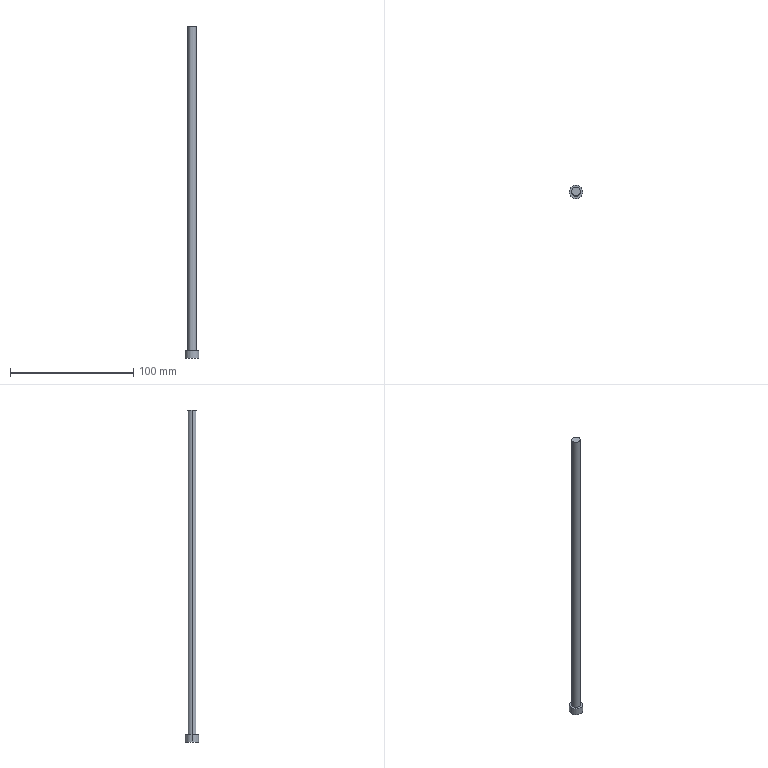Part | Creo | 1 solid | 7 faces | box 11 x 11 x 269.601 mm | volume 10715 mm3 | cylinder 4 | plane 3 | commonest cylinder face diameters 7 x2 11 x2
STEP:
#1=CARTESIAN_POINT('',(0.,0.,0.));
#2=DIRECTION('',(0.,0.,1.));
#3=DIRECTION('',(1.,0.,0.));
#4=AXIS2_PLACEMENT_3D('',#1,#2,#3);
#5=CARTESIAN_POINT('',(33.5,-43.5,-219.5));
#6=VERTEX_POINT('',#5);
#7=CARTESIAN_POINT('',(40.5,-43.5,-219.5));
#8=VERTEX_POINT('',#7);
#9=CARTESIAN_POINT('',(37.,-43.5,-219.5));
#10=DIRECTION('',(0.,0.,-1.));
#11=DIRECTION('',(-1.,0.,0.));
#12=AXIS2_PLACEMENT_3D('',#9,#10,#11);
#13=CIRCLE('',#12,3.5);
#14=EDGE_CURVE('',#6,#8,#13,.T.);
#15=ORIENTED_EDGE('',*,*,#14,.T.);
#16=CARTESIAN_POINT('',(40.5,-43.5,44.101));
#17=VERTEX_POINT('',#16);
#18=CARTESIAN_POINT('',(40.5,-43.5,44.101));
#19=DIRECTION('',(0.,0.,-1.));
#20=VECTOR('',#19,263.601);
#21=LINE('',#18,#20);
#22=EDGE_CURVE('',#17,#8,#21,.T.);
#23=ORIENTED_EDGE('',*,*,#22,.F.);
#24=CARTESIAN_POINT('',(33.5,-43.5,44.101));
#25=VERTEX_POINT('',#24);
#26=CARTESIAN_POINT('',(37.,-43.5,44.101));
#27=DIRECTION('',(0.,0.,1.));
#28=DIRECTION('',(1.,0.,0.));
#29=AXIS2_PLACEMENT_3D('',#26,#27,#28);
#30=CIRCLE('',#29,3.5);
#31=EDGE_CURVE('',#17,#25,#30,.T.);
#32=ORIENTED_EDGE('',*,*,#31,.T.);
#33=CARTESIAN_POINT('',(33.5,-43.5,44.101));
#34=DIRECTION('',(0.,0.,-1.));
#35=VECTOR('',#34,263.601);
#36=LINE('',#33,#35);
#37=EDGE_CURVE('',#25,#6,#36,.T.);
#38=ORIENTED_EDGE('',*,*,#37,.T.);
#39=EDGE_LOOP('',(#15,#23,#32,#38));
#40=FACE_OUTER_BOUND('',#39,.F.);
#41=CARTESIAN_POINT('',(37.,-43.5,125.91));
#42=DIRECTION('',(0.,0.,-1.));
#43=DIRECTION('',(-1.,0.,0.));
#44=AXIS2_PLACEMENT_3D('',#41,#42,#43);
#45=CYLINDRICAL_SURFACE('',#44,3.5);
#46=ADVANCED_FACE('',(#40),#45,.T.);
#47=CARTESIAN_POINT('',(31.5,-43.5,-219.5));
#48=VERTEX_POINT('',#47);
#49=CARTESIAN_POINT('',(42.5,-43.5,-219.5));
#50=VERTEX_POINT('',#49);
#51=CARTESIAN_POINT('',(37.,-43.5,-219.5));
#52=DIRECTION('',(0.,0.,1.));
#53=DIRECTION('',(-1.,0.,0.));
#54=AXIS2_PLACEMENT_3D('',#51,#52,#53);
#55=CIRCLE('',#54,5.5);
#56=EDGE_CURVE('',#48,#50,#55,.T.);
#57=ORIENTED_EDGE('',*,*,#56,.F.);
#58=CARTESIAN_POINT('',(37.,-43.5,-219.5));
#59=DIRECTION('',(0.,0.,1.));
#60=DIRECTION('',(1.,0.,0.));
#61=AXIS2_PLACEMENT_3D('',#58,#59,#60);
#62=CIRCLE('',#61,5.5);
#63=EDGE_CURVE('',#50,#48,#62,.T.);
#64=ORIENTED_EDGE('',*,*,#63,.F.);
#65=EDGE_LOOP('',(#57,#64));
#66=FACE_OUTER_BOUND('',#65,.F.);
#67=ORIENTED_EDGE('',*,*,#14,.F.);
#68=CARTESIAN_POINT('',(37.,-43.5,-219.5));
#69=DIRECTION('',(0.,0.,-1.));
#70=DIRECTION('',(1.,0.,0.));
#71=AXIS2_PLACEMENT_3D('',#68,#69,#70);
#72=CIRCLE('',#71,3.5);
#73=EDGE_CURVE('',#8,#6,#72,.T.);
#74=ORIENTED_EDGE('',*,*,#73,.F.);
#75=EDGE_LOOP('',(#67,#74));
#76=FACE_BOUND('',#75,.F.);
#77=CARTESIAN_POINT('',(0.,26.,-219.5));
#78=DIRECTION('',(0.,0.,-1.));
#79=DIRECTION('',(-1.,0.,0.));
#80=AXIS2_PLACEMENT_3D('',#77,#78,#79);
#81=PLANE('',#80);
#82=ADVANCED_FACE('',(#66,#76),#81,.F.);
#83=CARTESIAN_POINT('',(42.5,-43.5,-225.5));
#84=VERTEX_POINT('',#83);
#85=CARTESIAN_POINT('',(31.5,-43.5,-225.5));
#86=VERTEX_POINT('',#85);
#87=CARTESIAN_POINT('',(37.,-43.5,-225.5));
#88=DIRECTION('',(0.,0.,-1.));
#89=DIRECTION('',(1.,0.,0.));
#90=AXIS2_PLACEMENT_3D('',#87,#88,#89);
#91=CIRCLE('',#90,5.5);
#92=EDGE_CURVE('',#84,#86,#91,.T.);
#93=ORIENTED_EDGE('',*,*,#92,.T.);
#94=CARTESIAN_POINT('',(31.5,-43.5,-225.5));
#95=DIRECTION('',(0.,0.,1.));
#96=VECTOR('',#95,6.);
#97=LINE('',#94,#96);
#98=EDGE_CURVE('',#86,#48,#97,.T.);
#99=ORIENTED_EDGE('',*,*,#98,.T.);
#100=ORIENTED_EDGE('',*,*,#56,.T.);
#101=CARTESIAN_POINT('',(42.5,-43.5,-225.5));
#102=DIRECTION('',(0.,0.,1.));
#103=VECTOR('',#102,6.);
#104=LINE('',#101,#103);
#105=EDGE_CURVE('',#84,#50,#104,.T.);
#106=ORIENTED_EDGE('',*,*,#105,.F.);
#107=EDGE_LOOP('',(#93,#99,#100,#106));
#108=FACE_OUTER_BOUND('',#107,.F.);
#109=CARTESIAN_POINT('',(37.,-43.5,-225.5));
#110=DIRECTION('',(0.,0.,1.));
#111=DIRECTION('',(1.,0.,0.));
#112=AXIS2_PLACEMENT_3D('',#109,#110,#111);
#113=CYLINDRICAL_SURFACE('',#112,5.5);
#114=ADVANCED_FACE('',(#108),#113,.T.);
#115=CARTESIAN_POINT('',(37.,-43.5,-225.5));
#116=DIRECTION('',(0.,0.,-1.));
#117=DIRECTION('',(-1.,0.,0.));
#118=AXIS2_PLACEMENT_3D('',#115,#116,#117);
#119=CIRCLE('',#118,5.5);
#120=EDGE_CURVE('',#86,#84,#119,.T.);
#121=ORIENTED_EDGE('',*,*,#120,.F.);
#122=ORIENTED_EDGE('',*,*,#92,.F.);
#123=EDGE_LOOP('',(#121,#122));
#124=FACE_OUTER_BOUND('',#123,.F.);
#125=CARTESIAN_POINT('',(0.,26.,-225.5));
#126=DIRECTION('',(0.,0.,-1.));
#127=DIRECTION('',(-1.,0.,0.));
#128=AXIS2_PLACEMENT_3D('',#125,#126,#127);
#129=PLANE('',#128);
#130=ADVANCED_FACE('',(#124),#129,.T.);
#131=ORIENTED_EDGE('',*,*,#120,.T.);
#132=ORIENTED_EDGE('',*,*,#105,.T.);
#133=ORIENTED_EDGE('',*,*,#63,.T.);
#134=ORIENTED_EDGE('',*,*,#98,.F.);
#135=EDGE_LOOP('',(#131,#132,#133,#134));
#136=FACE_OUTER_BOUND('',#135,.F.);
#137=CARTESIAN_POINT('',(37.,-43.5,-225.5));
#138=DIRECTION('',(0.,0.,1.));
#139=DIRECTION('',(1.,0.,0.));
#140=AXIS2_PLACEMENT_3D('',#137,#138,#139);
#141=CYLINDRICAL_SURFACE('',#140,5.5);
#142=ADVANCED_FACE('',(#136),#141,.T.);
#143=ORIENTED_EDGE('',*,*,#73,.T.);
#144=ORIENTED_EDGE('',*,*,#37,.F.);
#145=CARTESIAN_POINT('',(37.,-43.5,44.101));
#146=DIRECTION('',(0.,0.,1.));
#147=DIRECTION('',(-1.,0.,0.));
#148=AXIS2_PLACEMENT_3D('',#145,#146,#147);
#149=CIRCLE('',#148,3.5);
#150=EDGE_CURVE('',#25,#17,#149,.T.);
#151=ORIENTED_EDGE('',*,*,#150,.T.);
#152=ORIENTED_EDGE('',*,*,#22,.T.);
#153=EDGE_LOOP('',(#143,#144,#151,#152));
#154=FACE_OUTER_BOUND('',#153,.F.);
#155=CARTESIAN_POINT('',(37.,-43.5,125.91));
#156=DIRECTION('',(0.,0.,-1.));
#157=DIRECTION('',(-1.,0.,0.));
#158=AXIS2_PLACEMENT_3D('',#155,#156,#157);
#159=CYLINDRICAL_SURFACE('',#158,3.5);
#160=ADVANCED_FACE('',(#154),#159,.T.);
#161=ORIENTED_EDGE('',*,*,#31,.F.);
#162=ORIENTED_EDGE('',*,*,#150,.F.);
#163=EDGE_LOOP('',(#161,#162));
#164=FACE_OUTER_BOUND('',#163,.F.);
#165=CARTESIAN_POINT('',(31.263,28.082,44.101));
#166=DIRECTION('',(0.,0.,1.));
#167=DIRECTION('',(1.,0.,0.));
#168=AXIS2_PLACEMENT_3D('',#165,#166,#167);
#169=PLANE('',#168);
#170=ADVANCED_FACE('',(#164),#169,.T.);
#171=CLOSED_SHELL('',(#46,#82,#114,#130,#142,#160,#170));
#172=MANIFOLD_SOLID_BREP('',#171);
#173=(LENGTH_UNIT()NAMED_UNIT(*)SI_UNIT(.MILLI.,.METRE.));
#174=UNCERTAINTY_MEASURE_WITH_UNIT(LENGTH_MEASURE(0.027),#173,'','');
#175=(NAMED_UNIT(*)PLANE_ANGLE_UNIT()SI_UNIT($,.RADIAN.));
#176=PLANE_ANGLE_MEASURE_WITH_UNIT(PLANE_ANGLE_MEASURE(0.01745),#175);
#177=(CONVERSION_BASED_UNIT('DEGREE',#176)NAMED_UNIT(*)PLANE_ANGLE_UNIT());
#178=(NAMED_UNIT(*)SI_UNIT($,.STERADIAN.)SOLID_ANGLE_UNIT());
#179=(GEOMETRIC_REPRESENTATION_CONTEXT(3)GLOBAL_UNCERTAINTY_ASSIGNED_CONTEXT((#174))GLOBAL_UNIT_ASSIGNED_CONTEXT((#173,#177,#178))REPRESENTATION_CONTEXT('',''));
#180=ADVANCED_BREP_SHAPE_REPRESENTATION('',(#4,#172),#179);